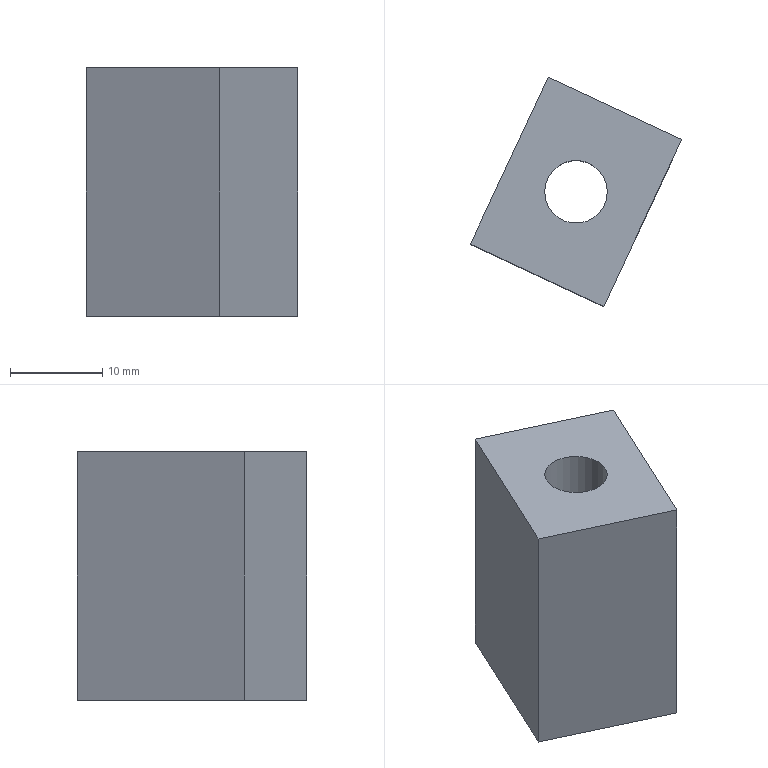Part | STEP file | gslz 2016.10.28-13_id1474_x_t | 1 solid | 9 faces | box 22.953 x 24.888 x 27 mm | volume 6892 mm3 | plane 7 | cylinder 2 | commonest cylinder face diameters 6.8 x1 12 x1
STEP:
#1=CARTESIAN_POINT('',(0.,0.,0.));
#2=DIRECTION('',(0.,0.,1.));
#3=DIRECTION('',(1.,0.,0.));
#4=AXIS2_PLACEMENT_3D('',#1,#2,#3);
#5=CARTESIAN_POINT('',(821.405,-311.945,-70.5));
#6=VERTEX_POINT('',#5);
#7=CARTESIAN_POINT('',(812.953,-330.071,-70.5));
#8=VERTEX_POINT('',#7);
#9=CARTESIAN_POINT('',(815.568,-324.462,-70.5));
#10=DIRECTION('',(-0.4226,-0.9063,0.));
#11=VECTOR('',#10,1.);
#12=LINE('',#9,#11);
#13=CARTESIAN_POINT('',(822.25,-310.132,-97.82));
#14=DIRECTION('',(-0.9063,0.4226,0.));
#15=DIRECTION('',(-0.4226,-0.9063,0.));
#16=AXIS2_PLACEMENT_3D('',#13,#14,#15);
#17=PLANE('',#16);
#18=CARTESIAN_POINT('',(15.812,27.32));
#19=DIRECTION('',(1.,0.));
#20=VECTOR('',#19,1.);
#21=LINE('',#18,#20);
#22=(GEOMETRIC_REPRESENTATION_CONTEXT(2)PARAMETRIC_REPRESENTATION_CONTEXT()REPRESENTATION_CONTEXT('',''));
#23=DEFINITIONAL_REPRESENTATION('',(#21),#22);
#24=PCURVE('',#17,#23);
#25=CARTESIAN_POINT('',(811.463,-322.548,-70.5));
#26=DIRECTION('',(0.,0.,1.));
#27=DIRECTION('',(-0.9397,-0.342,0.));
#28=AXIS2_PLACEMENT_3D('',#25,#26,#27);
#29=PLANE('',#28);
#30=CARTESIAN_POINT('',(-3.202,3.202));
#31=DIRECTION('',(0.7071,0.7071));
#32=VECTOR('',#31,1.);
#33=LINE('',#30,#32);
#34=(GEOMETRIC_REPRESENTATION_CONTEXT(2)PARAMETRIC_REPRESENTATION_CONTEXT()REPRESENTATION_CONTEXT('',''));
#35=DEFINITIONAL_REPRESENTATION('',(#33),#34);
#36=PCURVE('',#29,#35);
#37=SURFACE_CURVE('',#12,(#24,#36),.PCURVE_S1.);
#38=EDGE_CURVE('',#6,#8,#37,.T.);
#39=ORIENTED_EDGE('',*,*,#38,.F.);
#40=CARTESIAN_POINT('',(821.405,-311.945,-97.5));
#41=VERTEX_POINT('',#40);
#42=CARTESIAN_POINT('',(821.405,-311.945,-97.82));
#43=DIRECTION('',(0.,0.,1.));
#44=VECTOR('',#43,1.);
#45=LINE('',#42,#44);
#46=CARTESIAN_POINT('',(2.,0.));
#47=DIRECTION('',(0.,1.));
#48=VECTOR('',#47,1.);
#49=LINE('',#46,#48);
#50=(GEOMETRIC_REPRESENTATION_CONTEXT(2)PARAMETRIC_REPRESENTATION_CONTEXT()REPRESENTATION_CONTEXT('',''));
#51=DEFINITIONAL_REPRESENTATION('',(#49),#50);
#52=PCURVE('',#17,#51);
#53=CARTESIAN_POINT('',(839.531,-320.397,-97.82));
#54=DIRECTION('',(0.4226,0.9063,0.));
#55=DIRECTION('',(-0.9063,0.4226,0.));
#56=AXIS2_PLACEMENT_3D('',#53,#54,#55);
#57=PLANE('',#56);
#58=CARTESIAN_POINT('',(20.,0.));
#59=DIRECTION('',(0.,1.));
#60=VECTOR('',#59,1.);
#61=LINE('',#58,#60);
#62=(GEOMETRIC_REPRESENTATION_CONTEXT(2)PARAMETRIC_REPRESENTATION_CONTEXT()REPRESENTATION_CONTEXT('',''));
#63=DEFINITIONAL_REPRESENTATION('',(#61),#62);
#64=PCURVE('',#57,#63);
#65=SURFACE_CURVE('',#45,(#52,#64),.PCURVE_S1.);
#66=EDGE_CURVE('',#41,#6,#65,.T.);
#67=ORIENTED_EDGE('',*,*,#66,.F.);
#68=CARTESIAN_POINT('',(812.953,-330.071,-97.5));
#69=VERTEX_POINT('',#68);
#70=CARTESIAN_POINT('',(815.568,-324.462,-97.5));
#71=DIRECTION('',(-0.4226,-0.9063,0.));
#72=VECTOR('',#71,1.);
#73=LINE('',#70,#72);
#74=CARTESIAN_POINT('',(15.812,0.3195));
#75=DIRECTION('',(1.,0.));
#76=VECTOR('',#75,1.);
#77=LINE('',#74,#76);
#78=(GEOMETRIC_REPRESENTATION_CONTEXT(2)PARAMETRIC_REPRESENTATION_CONTEXT()REPRESENTATION_CONTEXT('',''));
#79=DEFINITIONAL_REPRESENTATION('',(#77),#78);
#80=PCURVE('',#17,#79);
#81=CARTESIAN_POINT('',(811.463,-322.548,-97.5));
#82=DIRECTION('',(0.,0.,1.));
#83=DIRECTION('',(-0.9397,-0.342,0.));
#84=AXIS2_PLACEMENT_3D('',#81,#82,#83);
#85=PLANE('',#84);
#86=CARTESIAN_POINT('',(-3.202,3.202));
#87=DIRECTION('',(0.7071,0.7071));
#88=VECTOR('',#87,1.);
#89=LINE('',#86,#88);
#90=(GEOMETRIC_REPRESENTATION_CONTEXT(2)PARAMETRIC_REPRESENTATION_CONTEXT()REPRESENTATION_CONTEXT('',''));
#91=DEFINITIONAL_REPRESENTATION('',(#89),#90);
#92=PCURVE('',#85,#91);
#93=SURFACE_CURVE('',#73,(#80,#92),.PCURVE_S1.);
#94=EDGE_CURVE('',#41,#69,#93,.T.);
#95=ORIENTED_EDGE('',*,*,#94,.T.);
#96=CARTESIAN_POINT('',(812.953,-330.071,-97.82));
#97=DIRECTION('',(0.,0.,1.));
#98=VECTOR('',#97,1.);
#99=LINE('',#96,#98);
#100=CARTESIAN_POINT('',(22.,0.));
#101=DIRECTION('',(0.,1.));
#102=VECTOR('',#101,1.);
#103=LINE('',#100,#102);
#104=(GEOMETRIC_REPRESENTATION_CONTEXT(2)PARAMETRIC_REPRESENTATION_CONTEXT()REPRESENTATION_CONTEXT('',''));
#105=DEFINITIONAL_REPRESENTATION('',(#103),#104);
#106=PCURVE('',#17,#105);
#107=CARTESIAN_POINT('',(809.327,-328.381,-97.82));
#108=DIRECTION('',(-0.4226,-0.9063,0.));
#109=DIRECTION('',(0.9063,-0.4226,0.));
#110=AXIS2_PLACEMENT_3D('',#107,#108,#109);
#111=PLANE('',#110);
#112=CARTESIAN_POINT('',(4.,0.));
#113=DIRECTION('',(0.,1.));
#114=VECTOR('',#113,1.);
#115=LINE('',#112,#114);
#116=(GEOMETRIC_REPRESENTATION_CONTEXT(2)PARAMETRIC_REPRESENTATION_CONTEXT()REPRESENTATION_CONTEXT('',''));
#117=DEFINITIONAL_REPRESENTATION('',(#115),#116);
#118=PCURVE('',#111,#117);
#119=SURFACE_CURVE('',#99,(#106,#118),.PCURVE_S1.);
#120=EDGE_CURVE('',#69,#8,#119,.T.);
#121=ORIENTED_EDGE('',*,*,#120,.T.);
#122=EDGE_LOOP('',(#39,#67,#95,#121));
#123=FACE_BOUND('',#122,.T.);
#124=ADVANCED_FACE('',(#123),#17,.T.);
#125=CARTESIAN_POINT('',(827.454,-336.833,-70.5));
#126=VERTEX_POINT('',#125);
#127=CARTESIAN_POINT('',(808.848,-328.157,-70.5));
#128=DIRECTION('',(0.9063,-0.4226,0.));
#129=VECTOR('',#128,1.);
#130=LINE('',#127,#129);
#131=CARTESIAN_POINT('',(-0.5289,27.32));
#132=DIRECTION('',(1.,0.));
#133=VECTOR('',#132,1.);
#134=LINE('',#131,#133);
#135=(GEOMETRIC_REPRESENTATION_CONTEXT(2)PARAMETRIC_REPRESENTATION_CONTEXT()REPRESENTATION_CONTEXT('',''));
#136=DEFINITIONAL_REPRESENTATION('',(#134),#135);
#137=PCURVE('',#111,#136);
#138=CARTESIAN_POINT('',(4.376,4.376));
#139=DIRECTION('',(-0.7071,0.7071));
#140=VECTOR('',#139,1.);
#141=LINE('',#138,#140);
#142=(GEOMETRIC_REPRESENTATION_CONTEXT(2)PARAMETRIC_REPRESENTATION_CONTEXT()REPRESENTATION_CONTEXT('',''));
#143=DEFINITIONAL_REPRESENTATION('',(#141),#142);
#144=PCURVE('',#29,#143);
#145=SURFACE_CURVE('',#130,(#137,#144),.PCURVE_S1.);
#146=EDGE_CURVE('',#8,#126,#145,.T.);
#147=ORIENTED_EDGE('',*,*,#146,.F.);
#148=ORIENTED_EDGE('',*,*,#120,.F.);
#149=CARTESIAN_POINT('',(827.454,-336.833,-97.5));
#150=VERTEX_POINT('',#149);
#151=CARTESIAN_POINT('',(808.848,-328.157,-97.5));
#152=DIRECTION('',(0.9063,-0.4226,0.));
#153=VECTOR('',#152,1.);
#154=LINE('',#151,#153);
#155=CARTESIAN_POINT('',(-0.5289,0.3195));
#156=DIRECTION('',(1.,0.));
#157=VECTOR('',#156,1.);
#158=LINE('',#155,#157);
#159=(GEOMETRIC_REPRESENTATION_CONTEXT(2)PARAMETRIC_REPRESENTATION_CONTEXT()REPRESENTATION_CONTEXT('',''));
#160=DEFINITIONAL_REPRESENTATION('',(#158),#159);
#161=PCURVE('',#111,#160);
#162=CARTESIAN_POINT('',(4.376,4.376));
#163=DIRECTION('',(-0.7071,0.7071));
#164=VECTOR('',#163,1.);
#165=LINE('',#162,#164);
#166=(GEOMETRIC_REPRESENTATION_CONTEXT(2)PARAMETRIC_REPRESENTATION_CONTEXT()REPRESENTATION_CONTEXT('',''));
#167=DEFINITIONAL_REPRESENTATION('',(#165),#166);
#168=PCURVE('',#85,#167);
#169=SURFACE_CURVE('',#154,(#161,#168),.PCURVE_S1.);
#170=EDGE_CURVE('',#69,#150,#169,.T.);
#171=ORIENTED_EDGE('',*,*,#170,.T.);
#172=CARTESIAN_POINT('',(827.454,-336.833,-97.82));
#173=DIRECTION('',(0.,0.,1.));
#174=VECTOR('',#173,1.);
#175=LINE('',#172,#174);
#176=CARTESIAN_POINT('',(20.,0.));
#177=DIRECTION('',(0.,1.));
#178=VECTOR('',#177,1.);
#179=LINE('',#176,#178);
#180=(GEOMETRIC_REPRESENTATION_CONTEXT(2)PARAMETRIC_REPRESENTATION_CONTEXT()REPRESENTATION_CONTEXT('',''));
#181=DEFINITIONAL_REPRESENTATION('',(#179),#180);
#182=PCURVE('',#111,#181);
#183=CARTESIAN_POINT('',(826.608,-338.646,-97.82));
#184=DIRECTION('',(0.9063,-0.4226,0.));
#185=DIRECTION('',(0.4226,0.9063,0.));
#186=AXIS2_PLACEMENT_3D('',#183,#184,#185);
#187=PLANE('',#186);
#188=CARTESIAN_POINT('',(2.,0.));
#189=DIRECTION('',(0.,1.));
#190=VECTOR('',#189,1.);
#191=LINE('',#188,#190);
#192=(GEOMETRIC_REPRESENTATION_CONTEXT(2)PARAMETRIC_REPRESENTATION_CONTEXT()REPRESENTATION_CONTEXT('',''));
#193=DEFINITIONAL_REPRESENTATION('',(#191),#192);
#194=PCURVE('',#187,#193);
#195=SURFACE_CURVE('',#175,(#182,#194),.PCURVE_S1.);
#196=EDGE_CURVE('',#150,#126,#195,.T.);
#197=ORIENTED_EDGE('',*,*,#196,.T.);
#198=EDGE_LOOP('',(#147,#148,#171,#197));
#199=FACE_BOUND('',#198,.T.);
#200=ADVANCED_FACE('',(#199),#111,.T.);
#201=CARTESIAN_POINT('',(835.906,-318.707,-70.5));
#202=VERTEX_POINT('',#201);
#203=CARTESIAN_POINT('',(830.069,-331.224,-70.5));
#204=DIRECTION('',(0.4226,0.9063,0.));
#205=VECTOR('',#204,1.);
#206=LINE('',#203,#205);
#207=CARTESIAN_POINT('',(8.188,27.32));
#208=DIRECTION('',(1.,0.));
#209=VECTOR('',#208,1.);
#210=LINE('',#207,#209);
#211=(GEOMETRIC_REPRESENTATION_CONTEXT(2)PARAMETRIC_REPRESENTATION_CONTEXT()REPRESENTATION_CONTEXT('',''));
#212=DEFINITIONAL_REPRESENTATION('',(#210),#211);
#213=PCURVE('',#187,#212);
#214=CARTESIAN_POINT('',(-14.516,14.516));
#215=DIRECTION('',(-0.7071,-0.7071));
#216=VECTOR('',#215,1.);
#217=LINE('',#214,#216);
#218=(GEOMETRIC_REPRESENTATION_CONTEXT(2)PARAMETRIC_REPRESENTATION_CONTEXT()REPRESENTATION_CONTEXT('',''));
#219=DEFINITIONAL_REPRESENTATION('',(#217),#218);
#220=PCURVE('',#29,#219);
#221=SURFACE_CURVE('',#206,(#213,#220),.PCURVE_S1.);
#222=EDGE_CURVE('',#126,#202,#221,.T.);
#223=ORIENTED_EDGE('',*,*,#222,.F.);
#224=ORIENTED_EDGE('',*,*,#196,.F.);
#225=CARTESIAN_POINT('',(835.906,-318.707,-97.5));
#226=VERTEX_POINT('',#225);
#227=CARTESIAN_POINT('',(830.069,-331.224,-97.5));
#228=DIRECTION('',(0.4226,0.9063,0.));
#229=VECTOR('',#228,1.);
#230=LINE('',#227,#229);
#231=CARTESIAN_POINT('',(8.188,0.3195));
#232=DIRECTION('',(1.,0.));
#233=VECTOR('',#232,1.);
#234=LINE('',#231,#233);
#235=(GEOMETRIC_REPRESENTATION_CONTEXT(2)PARAMETRIC_REPRESENTATION_CONTEXT()REPRESENTATION_CONTEXT('',''));
#236=DEFINITIONAL_REPRESENTATION('',(#234),#235);
#237=PCURVE('',#187,#236);
#238=CARTESIAN_POINT('',(-14.516,14.516));
#239=DIRECTION('',(-0.7071,-0.7071));
#240=VECTOR('',#239,1.);
#241=LINE('',#238,#240);
#242=(GEOMETRIC_REPRESENTATION_CONTEXT(2)PARAMETRIC_REPRESENTATION_CONTEXT()REPRESENTATION_CONTEXT('',''));
#243=DEFINITIONAL_REPRESENTATION('',(#241),#242);
#244=PCURVE('',#85,#243);
#245=SURFACE_CURVE('',#230,(#237,#244),.PCURVE_S1.);
#246=EDGE_CURVE('',#150,#226,#245,.T.);
#247=ORIENTED_EDGE('',*,*,#246,.T.);
#248=CARTESIAN_POINT('',(835.906,-318.707,-97.82));
#249=DIRECTION('',(0.,0.,1.));
#250=VECTOR('',#249,1.);
#251=LINE('',#248,#250);
#252=CARTESIAN_POINT('',(22.,0.));
#253=DIRECTION('',(0.,1.));
#254=VECTOR('',#253,1.);
#255=LINE('',#252,#254);
#256=(GEOMETRIC_REPRESENTATION_CONTEXT(2)PARAMETRIC_REPRESENTATION_CONTEXT()REPRESENTATION_CONTEXT('',''));
#257=DEFINITIONAL_REPRESENTATION('',(#255),#256);
#258=PCURVE('',#187,#257);
#259=CARTESIAN_POINT('',(4.,0.));
#260=DIRECTION('',(0.,1.));
#261=VECTOR('',#260,1.);
#262=LINE('',#259,#261);
#263=(GEOMETRIC_REPRESENTATION_CONTEXT(2)PARAMETRIC_REPRESENTATION_CONTEXT()REPRESENTATION_CONTEXT('',''));
#264=DEFINITIONAL_REPRESENTATION('',(#262),#263);
#265=PCURVE('',#57,#264);
#266=SURFACE_CURVE('',#251,(#258,#265),.PCURVE_S1.);
#267=EDGE_CURVE('',#226,#202,#266,.T.);
#268=ORIENTED_EDGE('',*,*,#267,.T.);
#269=EDGE_LOOP('',(#223,#224,#247,#268));
#270=FACE_BOUND('',#269,.T.);
#271=ADVANCED_FACE('',(#270),#187,.T.);
#272=CARTESIAN_POINT('',(817.3,-310.031,-70.5));
#273=DIRECTION('',(-0.9063,0.4226,0.));
#274=VECTOR('',#273,1.);
#275=LINE('',#272,#274);
#276=CARTESIAN_POINT('',(24.529,27.32));
#277=DIRECTION('',(1.,0.));
#278=VECTOR('',#277,1.);
#279=LINE('',#276,#278);
#280=(GEOMETRIC_REPRESENTATION_CONTEXT(2)PARAMETRIC_REPRESENTATION_CONTEXT()REPRESENTATION_CONTEXT('',''));
#281=DEFINITIONAL_REPRESENTATION('',(#279),#280);
#282=PCURVE('',#57,#281);
#283=CARTESIAN_POINT('',(-9.766,-9.766));
#284=DIRECTION('',(0.7071,-0.7071));
#285=VECTOR('',#284,1.);
#286=LINE('',#283,#285);
#287=(GEOMETRIC_REPRESENTATION_CONTEXT(2)PARAMETRIC_REPRESENTATION_CONTEXT()REPRESENTATION_CONTEXT('',''));
#288=DEFINITIONAL_REPRESENTATION('',(#286),#287);
#289=PCURVE('',#29,#288);
#290=SURFACE_CURVE('',#275,(#282,#289),.PCURVE_S1.);
#291=EDGE_CURVE('',#202,#6,#290,.T.);
#292=ORIENTED_EDGE('',*,*,#291,.F.);
#293=ORIENTED_EDGE('',*,*,#267,.F.);
#294=CARTESIAN_POINT('',(817.3,-310.031,-97.5));
#295=DIRECTION('',(-0.9063,0.4226,0.));
#296=VECTOR('',#295,1.);
#297=LINE('',#294,#296);
#298=CARTESIAN_POINT('',(24.529,0.3195));
#299=DIRECTION('',(1.,0.));
#300=VECTOR('',#299,1.);
#301=LINE('',#298,#300);
#302=(GEOMETRIC_REPRESENTATION_CONTEXT(2)PARAMETRIC_REPRESENTATION_CONTEXT()REPRESENTATION_CONTEXT('',''));
#303=DEFINITIONAL_REPRESENTATION('',(#301),#302);
#304=PCURVE('',#57,#303);
#305=CARTESIAN_POINT('',(-9.766,-9.766));
#306=DIRECTION('',(0.7071,-0.7071));
#307=VECTOR('',#306,1.);
#308=LINE('',#305,#307);
#309=(GEOMETRIC_REPRESENTATION_CONTEXT(2)PARAMETRIC_REPRESENTATION_CONTEXT()REPRESENTATION_CONTEXT('',''));
#310=DEFINITIONAL_REPRESENTATION('',(#308),#309);
#311=PCURVE('',#85,#310);
#312=SURFACE_CURVE('',#297,(#304,#311),.PCURVE_S1.);
#313=EDGE_CURVE('',#226,#41,#312,.T.);
#314=ORIENTED_EDGE('',*,*,#313,.T.);
#315=ORIENTED_EDGE('',*,*,#66,.T.);
#316=EDGE_LOOP('',(#292,#293,#314,#315));
#317=FACE_BOUND('',#316,.T.);
#318=ADVANCED_FACE('',(#317),#57,.T.);
#319=CARTESIAN_POINT('',(830.429,-324.389,-97.5));
#320=VERTEX_POINT('',#319);
#321=CARTESIAN_POINT('',(824.429,-324.389,-97.5));
#322=DIRECTION('',(0.,0.,1.));
#323=DIRECTION('',(1.,0.,0.));
#324=AXIS2_PLACEMENT_3D('',#321,#322,#323);
#325=CIRCLE('',#324,6.);
#326=CARTESIAN_POINT('',(-11.554,6.164));
#327=DIRECTION('',(-0.9397,0.342));
#328=AXIS2_PLACEMENT_2D('',#326,#327);
#329=CIRCLE('',#328,6.);
#330=(GEOMETRIC_REPRESENTATION_CONTEXT(2)PARAMETRIC_REPRESENTATION_CONTEXT()REPRESENTATION_CONTEXT('',''));
#331=DEFINITIONAL_REPRESENTATION('',(#329),#330);
#332=PCURVE('',#85,#331);
#333=CARTESIAN_POINT('',(824.429,-324.389,-97.82));
#334=DIRECTION('',(0.,0.,1.));
#335=DIRECTION('',(0.8909,-0.4543,0.));
#336=AXIS2_PLACEMENT_3D('',#333,#334,#335);
#337=CYLINDRICAL_SURFACE('',#336,6.);
#338=CARTESIAN_POINT('',(0.4716,0.3195));
#339=DIRECTION('',(1.,0.));
#340=VECTOR('',#339,1.);
#341=LINE('',#338,#340);
#342=(GEOMETRIC_REPRESENTATION_CONTEXT(2)PARAMETRIC_REPRESENTATION_CONTEXT()REPRESENTATION_CONTEXT('',''));
#343=DEFINITIONAL_REPRESENTATION('',(#341),#342);
#344=PCURVE('',#337,#343);
#345=SURFACE_CURVE('',#325,(#332,#344),.PCURVE_S1.);
#346=EDGE_CURVE('',#320,#320,#345,.T.);
#347=ORIENTED_EDGE('',*,*,#346,.T.);
#348=EDGE_LOOP('',(#347));
#349=FACE_BOUND('',#348,.T.);
#350=ORIENTED_EDGE('',*,*,#94,.F.);
#351=ORIENTED_EDGE('',*,*,#313,.F.);
#352=ORIENTED_EDGE('',*,*,#246,.F.);
#353=ORIENTED_EDGE('',*,*,#170,.F.);
#354=EDGE_LOOP('',(#350,#351,#352,#353));
#355=FACE_BOUND('',#354,.T.);
#356=ADVANCED_FACE('',(#349,#355),#85,.F.);
#357=CARTESIAN_POINT('',(827.829,-324.389,-70.5));
#358=VERTEX_POINT('',#357);
#359=CARTESIAN_POINT('',(824.429,-324.389,-70.5));
#360=DIRECTION('',(0.,0.,1.));
#361=DIRECTION('',(1.,0.,0.));
#362=AXIS2_PLACEMENT_3D('',#359,#360,#361);
#363=CIRCLE('',#362,3.4);
#364=CARTESIAN_POINT('',(-11.554,6.164));
#365=DIRECTION('',(-0.9397,0.342));
#366=AXIS2_PLACEMENT_2D('',#364,#365);
#367=CIRCLE('',#366,3.4);
#368=(GEOMETRIC_REPRESENTATION_CONTEXT(2)PARAMETRIC_REPRESENTATION_CONTEXT()REPRESENTATION_CONTEXT('',''));
#369=DEFINITIONAL_REPRESENTATION('',(#367),#368);
#370=PCURVE('',#29,#369);
#371=CARTESIAN_POINT('',(824.429,-324.389,-47.82));
#372=DIRECTION('',(0.,0.,1.));
#373=DIRECTION('',(0.8909,-0.4543,0.));
#374=AXIS2_PLACEMENT_3D('',#371,#372,#373);
#375=CYLINDRICAL_SURFACE('',#374,3.4);
#376=CARTESIAN_POINT('',(0.4716,-22.68));
#377=DIRECTION('',(1.,0.));
#378=VECTOR('',#377,1.);
#379=LINE('',#376,#378);
#380=(GEOMETRIC_REPRESENTATION_CONTEXT(2)PARAMETRIC_REPRESENTATION_CONTEXT()REPRESENTATION_CONTEXT('',''));
#381=DEFINITIONAL_REPRESENTATION('',(#379),#380);
#382=PCURVE('',#375,#381);
#383=SURFACE_CURVE('',#363,(#370,#382),.PCURVE_S1.);
#384=EDGE_CURVE('',#358,#358,#383,.T.);
#385=ORIENTED_EDGE('',*,*,#384,.F.);
#386=EDGE_LOOP('',(#385));
#387=FACE_BOUND('',#386,.T.);
#388=ORIENTED_EDGE('',*,*,#38,.T.);
#389=ORIENTED_EDGE('',*,*,#146,.T.);
#390=ORIENTED_EDGE('',*,*,#222,.T.);
#391=ORIENTED_EDGE('',*,*,#291,.T.);
#392=EDGE_LOOP('',(#388,#389,#390,#391));
#393=FACE_BOUND('',#392,.T.);
#394=ADVANCED_FACE('',(#387,#393),#29,.T.);
#395=ORIENTED_EDGE('',*,*,#384,.F.);
#396=CARTESIAN_POINT('',(827.829,-324.389,-87.5));
#397=VERTEX_POINT('',#396);
#398=CARTESIAN_POINT('',(827.829,-324.389,-87.5));
#399=CARTESIAN_POINT('',(827.829,-324.389,-70.5));
#400=B_SPLINE_CURVE_WITH_KNOTS('',1,(#398,#399),.UNSPECIFIED.,.F.,.F.,(2,2),(-39.68,-22.68),.PIECEWISE_BEZIER_KNOTS.);
#401=CARTESIAN_POINT('',(0.4716,0.));
#402=DIRECTION('',(0.,1.));
#403=VECTOR('',#402,1.);
#404=LINE('',#401,#403);
#405=(GEOMETRIC_REPRESENTATION_CONTEXT(2)PARAMETRIC_REPRESENTATION_CONTEXT()REPRESENTATION_CONTEXT('',''));
#406=DEFINITIONAL_REPRESENTATION('',(#404),#405);
#407=PCURVE('',#375,#406);
#408=CARTESIAN_POINT('',(6.755,0.));
#409=DIRECTION('',(0.,1.));
#410=VECTOR('',#409,1.);
#411=LINE('',#408,#410);
#412=(GEOMETRIC_REPRESENTATION_CONTEXT(2)PARAMETRIC_REPRESENTATION_CONTEXT()REPRESENTATION_CONTEXT('',''));
#413=DEFINITIONAL_REPRESENTATION('',(#411),#412);
#414=PCURVE('',#375,#413);
#415=SEAM_CURVE('',#400,(#407,#414),.PCURVE_S1.);
#416=EDGE_CURVE('',#397,#358,#415,.T.);
#417=ORIENTED_EDGE('',*,*,#416,.F.);
#418=CARTESIAN_POINT('',(824.429,-324.389,-87.5));
#419=DIRECTION('',(0.,0.,1.));
#420=DIRECTION('',(1.,0.,0.));
#421=AXIS2_PLACEMENT_3D('',#418,#419,#420);
#422=CIRCLE('',#421,3.4);
#423=CARTESIAN_POINT('',(0.4716,-39.68));
#424=DIRECTION('',(1.,0.));
#425=VECTOR('',#424,1.);
#426=LINE('',#423,#425);
#427=(GEOMETRIC_REPRESENTATION_CONTEXT(2)PARAMETRIC_REPRESENTATION_CONTEXT()REPRESENTATION_CONTEXT('',''));
#428=DEFINITIONAL_REPRESENTATION('',(#426),#427);
#429=PCURVE('',#375,#428);
#430=CARTESIAN_POINT('',(811.463,-322.548,-87.5));
#431=DIRECTION('',(0.,0.,1.));
#432=DIRECTION('',(-0.9397,-0.342,0.));
#433=AXIS2_PLACEMENT_3D('',#430,#431,#432);
#434=PLANE('',#433);
#435=CARTESIAN_POINT('',(-11.554,6.164));
#436=DIRECTION('',(-0.9397,0.342));
#437=AXIS2_PLACEMENT_2D('',#435,#436);
#438=CIRCLE('',#437,3.4);
#439=(GEOMETRIC_REPRESENTATION_CONTEXT(2)PARAMETRIC_REPRESENTATION_CONTEXT()REPRESENTATION_CONTEXT('',''));
#440=DEFINITIONAL_REPRESENTATION('',(#438),#439);
#441=PCURVE('',#434,#440);
#442=SURFACE_CURVE('',#422,(#429,#441),.PCURVE_S1.);
#443=EDGE_CURVE('',#397,#397,#442,.T.);
#444=ORIENTED_EDGE('',*,*,#443,.T.);
#445=ORIENTED_EDGE('',*,*,#416,.T.);
#446=EDGE_LOOP('',(#395,#417,#444,#445));
#447=FACE_BOUND('',#446,.F.);
#448=ADVANCED_FACE('',(#447),#375,.F.);
#449=ORIENTED_EDGE('',*,*,#443,.T.);
#450=EDGE_LOOP('',(#449));
#451=FACE_BOUND('',#450,.T.);
#452=CARTESIAN_POINT('',(830.429,-324.389,-87.5));
#453=VERTEX_POINT('',#452);
#454=CARTESIAN_POINT('',(824.429,-324.389,-87.5));
#455=DIRECTION('',(0.,0.,1.));
#456=DIRECTION('',(1.,0.,0.));
#457=AXIS2_PLACEMENT_3D('',#454,#455,#456);
#458=CIRCLE('',#457,6.);
#459=CARTESIAN_POINT('',(-11.554,6.164));
#460=DIRECTION('',(-0.9397,0.342));
#461=AXIS2_PLACEMENT_2D('',#459,#460);
#462=CIRCLE('',#461,6.);
#463=(GEOMETRIC_REPRESENTATION_CONTEXT(2)PARAMETRIC_REPRESENTATION_CONTEXT()REPRESENTATION_CONTEXT('',''));
#464=DEFINITIONAL_REPRESENTATION('',(#462),#463);
#465=PCURVE('',#434,#464);
#466=CARTESIAN_POINT('',(0.4716,10.32));
#467=DIRECTION('',(1.,0.));
#468=VECTOR('',#467,1.);
#469=LINE('',#466,#468);
#470=(GEOMETRIC_REPRESENTATION_CONTEXT(2)PARAMETRIC_REPRESENTATION_CONTEXT()REPRESENTATION_CONTEXT('',''));
#471=DEFINITIONAL_REPRESENTATION('',(#469),#470);
#472=PCURVE('',#337,#471);
#473=SURFACE_CURVE('',#458,(#465,#472),.PCURVE_S1.);
#474=EDGE_CURVE('',#453,#453,#473,.T.);
#475=ORIENTED_EDGE('',*,*,#474,.F.);
#476=EDGE_LOOP('',(#475));
#477=FACE_BOUND('',#476,.T.);
#478=ADVANCED_FACE('',(#451,#477),#434,.F.);
#479=ORIENTED_EDGE('',*,*,#474,.F.);
#480=CARTESIAN_POINT('',(830.429,-324.389,-97.5));
#481=CARTESIAN_POINT('',(830.429,-324.389,-87.5));
#482=B_SPLINE_CURVE_WITH_KNOTS('',1,(#480,#481),.UNSPECIFIED.,.F.,.F.,(2,2),(0.3195,10.32),.PIECEWISE_BEZIER_KNOTS.);
#483=CARTESIAN_POINT('',(0.4716,0.));
#484=DIRECTION('',(0.,1.));
#485=VECTOR('',#484,1.);
#486=LINE('',#483,#485);
#487=(GEOMETRIC_REPRESENTATION_CONTEXT(2)PARAMETRIC_REPRESENTATION_CONTEXT()REPRESENTATION_CONTEXT('',''));
#488=DEFINITIONAL_REPRESENTATION('',(#486),#487);
#489=PCURVE('',#337,#488);
#490=CARTESIAN_POINT('',(6.755,0.));
#491=DIRECTION('',(0.,1.));
#492=VECTOR('',#491,1.);
#493=LINE('',#490,#492);
#494=(GEOMETRIC_REPRESENTATION_CONTEXT(2)PARAMETRIC_REPRESENTATION_CONTEXT()REPRESENTATION_CONTEXT('',''));
#495=DEFINITIONAL_REPRESENTATION('',(#493),#494);
#496=PCURVE('',#337,#495);
#497=SEAM_CURVE('',#482,(#489,#496),.PCURVE_S1.);
#498=EDGE_CURVE('',#320,#453,#497,.T.);
#499=ORIENTED_EDGE('',*,*,#498,.F.);
#500=ORIENTED_EDGE('',*,*,#346,.T.);
#501=ORIENTED_EDGE('',*,*,#498,.T.);
#502=EDGE_LOOP('',(#479,#499,#500,#501));
#503=FACE_BOUND('',#502,.F.);
#504=ADVANCED_FACE('',(#503),#337,.F.);
#505=CLOSED_SHELL('',(#124,#200,#271,#318,#356,#394,#448,#478,#504));
#506=MANIFOLD_SOLID_BREP('',#505);
#507=(LENGTH_UNIT()NAMED_UNIT(*)SI_UNIT(.MILLI.,.METRE.));
#508=UNCERTAINTY_MEASURE_WITH_UNIT(LENGTH_MEASURE(0.000002),#507,'','');
#509=(NAMED_UNIT(*)PLANE_ANGLE_UNIT()SI_UNIT($,.RADIAN.));
#510=(NAMED_UNIT(*)SI_UNIT($,.STERADIAN.)SOLID_ANGLE_UNIT());
#511=(GEOMETRIC_REPRESENTATION_CONTEXT(3)GLOBAL_UNCERTAINTY_ASSIGNED_CONTEXT((#508))GLOBAL_UNIT_ASSIGNED_CONTEXT((#507,#509,#510))REPRESENTATION_CONTEXT('',''));
#512=ADVANCED_BREP_SHAPE_REPRESENTATION('',(#4,#506),#511);